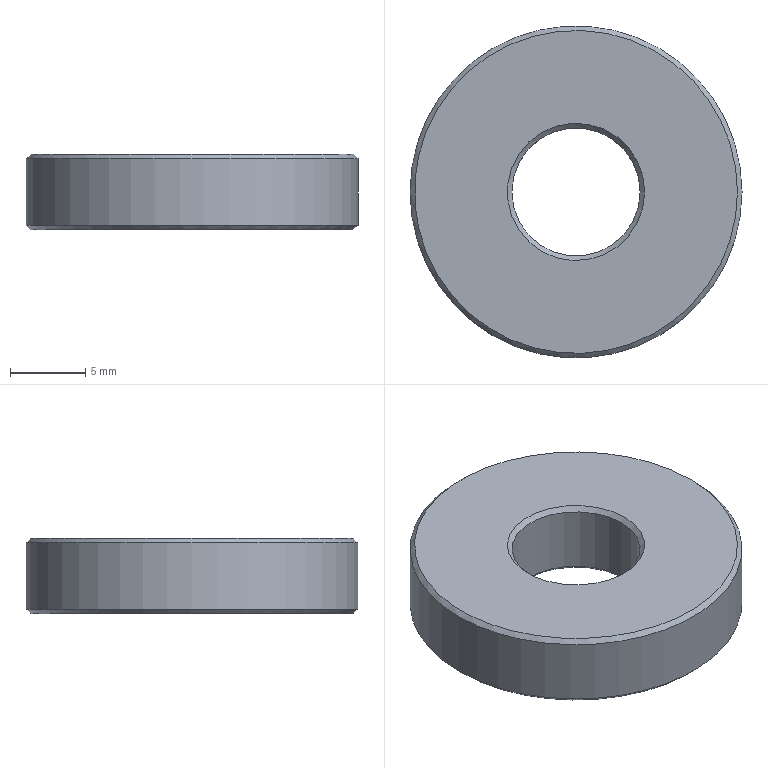Part | STEP file | 1 solid | 8 faces | box 22 x 22 x 5 mm | volume 1608 mm3 | cone 4 | plane 2 | cylinder 2 | commonest cylinder face diameters 8.5 x1 22 x1
STEP:
#1=CARTESIAN_POINT('',(0.,0.,0.));
#2=DIRECTION('',(0.,0.,1.));
#3=DIRECTION('',(1.,0.,0.));
#4=AXIS2_PLACEMENT_3D('',#1,#2,#3);
#5=CARTESIAN_POINT('',(1433.797,497.48,48.619));
#6=VERTEX_POINT('',#5);
#7=CARTESIAN_POINT('',(1429.247,497.48,48.619));
#8=DIRECTION('',(0.,0.,-1.));
#9=DIRECTION('',(1.,0.,0.));
#10=AXIS2_PLACEMENT_3D('',#7,#8,#9);
#11=CIRCLE('',#10,4.55);
#12=CARTESIAN_POINT('',(1429.247,497.48,48.619));
#13=DIRECTION('',(0.,0.,1.));
#14=DIRECTION('',(1.,0.,0.));
#15=AXIS2_PLACEMENT_3D('',#12,#13,#14);
#16=PLANE('',#15);
#17=CARTESIAN_POINT('',(4.55,0.));
#18=CARTESIAN_POINT('',(4.55,-7.881));
#19=CARTESIAN_POINT('',(-2.275,-3.94));
#20=CARTESIAN_POINT('',(-9.1,0.));
#21=CARTESIAN_POINT('',(-2.275,3.94));
#22=CARTESIAN_POINT('',(4.55,7.881));
#23=CARTESIAN_POINT('',(4.55,0.));
#24=(BOUNDED_CURVE()B_SPLINE_CURVE(2,(#17,#18,#19,#20,#21,#22,#23),.UNSPECIFIED.,.T.,.F.)B_SPLINE_CURVE_WITH_KNOTS((1,2,2,2,2,1),(-2.094,0.,2.094,4.189,6.283,8.378),.UNSPECIFIED.)CURVE()GEOMETRIC_REPRESENTATION_ITEM()RATIONAL_B_SPLINE_CURVE((1.,0.5,1.,0.5,1.,0.5,1.))REPRESENTATION_ITEM(''));
#25=(GEOMETRIC_REPRESENTATION_CONTEXT(2)PARAMETRIC_REPRESENTATION_CONTEXT()REPRESENTATION_CONTEXT('',''));
#26=DEFINITIONAL_REPRESENTATION('',(#24),#25);
#27=PCURVE('',#16,#26);
#28=CARTESIAN_POINT('',(1429.247,497.48,48.619));
#29=DIRECTION('',(0.,0.,1.));
#30=DIRECTION('',(1.,0.,0.));
#31=AXIS2_PLACEMENT_3D('',#28,#29,#30);
#32=CONICAL_SURFACE('',#31,4.55,0.7854);
#33=CARTESIAN_POINT('',(6.283,0.));
#34=DIRECTION('',(-1.,0.));
#35=VECTOR('',#34,1.);
#36=LINE('',#33,#35);
#37=(GEOMETRIC_REPRESENTATION_CONTEXT(2)PARAMETRIC_REPRESENTATION_CONTEXT()REPRESENTATION_CONTEXT('',''));
#38=DEFINITIONAL_REPRESENTATION('',(#36),#37);
#39=PCURVE('',#32,#38);
#40=SURFACE_CURVE('',#11,(#27,#39),.PCURVE_S1.);
#41=EDGE_CURVE('',#6,#6,#40,.T.);
#42=ORIENTED_EDGE('',*,*,#41,.T.);
#43=EDGE_LOOP('',(#42));
#44=FACE_BOUND('',#43,.T.);
#45=CARTESIAN_POINT('',(1439.947,497.48,48.619));
#46=VERTEX_POINT('',#45);
#47=CARTESIAN_POINT('',(1429.247,497.48,48.619));
#48=DIRECTION('',(0.,0.,1.));
#49=DIRECTION('',(1.,0.,0.));
#50=AXIS2_PLACEMENT_3D('',#47,#48,#49);
#51=CIRCLE('',#50,10.7);
#52=CARTESIAN_POINT('',(0.,0.));
#53=DIRECTION('',(1.,0.));
#54=AXIS2_PLACEMENT_2D('',#52,#53);
#55=CIRCLE('',#54,10.7);
#56=(GEOMETRIC_REPRESENTATION_CONTEXT(2)PARAMETRIC_REPRESENTATION_CONTEXT()REPRESENTATION_CONTEXT('',''));
#57=DEFINITIONAL_REPRESENTATION('',(#55),#56);
#58=PCURVE('',#16,#57);
#59=CARTESIAN_POINT('',(1429.247,497.48,48.619));
#60=DIRECTION('',(0.,0.,-1.));
#61=DIRECTION('',(-1.,0.,0.));
#62=AXIS2_PLACEMENT_3D('',#59,#60,#61);
#63=CONICAL_SURFACE('',#62,10.7,0.7854);
#64=CARTESIAN_POINT('',(9.425,0.));
#65=DIRECTION('',(-1.,0.));
#66=VECTOR('',#65,1.);
#67=LINE('',#64,#66);
#68=(GEOMETRIC_REPRESENTATION_CONTEXT(2)PARAMETRIC_REPRESENTATION_CONTEXT()REPRESENTATION_CONTEXT('',''));
#69=DEFINITIONAL_REPRESENTATION('',(#67),#68);
#70=PCURVE('',#63,#69);
#71=SURFACE_CURVE('',#51,(#58,#70),.PCURVE_S1.);
#72=EDGE_CURVE('',#46,#46,#71,.T.);
#73=ORIENTED_EDGE('',*,*,#72,.T.);
#74=EDGE_LOOP('',(#73));
#75=FACE_BOUND('',#74,.T.);
#76=ADVANCED_FACE('',(#44,#75),#16,.T.);
#77=CARTESIAN_POINT('',(1424.697,497.48,43.619));
#78=VERTEX_POINT('',#77);
#79=CARTESIAN_POINT('',(1429.247,497.48,43.619));
#80=DIRECTION('',(0.,0.,1.));
#81=DIRECTION('',(-1.,0.,0.));
#82=AXIS2_PLACEMENT_3D('',#79,#80,#81);
#83=CIRCLE('',#82,4.55);
#84=CARTESIAN_POINT('',(1429.247,497.48,43.619));
#85=DIRECTION('',(0.,0.,-1.));
#86=DIRECTION('',(-1.,0.,0.));
#87=AXIS2_PLACEMENT_3D('',#84,#85,#86);
#88=PLANE('',#87);
#89=CARTESIAN_POINT('',(4.55,0.));
#90=CARTESIAN_POINT('',(4.55,-7.881));
#91=CARTESIAN_POINT('',(-2.275,-3.94));
#92=CARTESIAN_POINT('',(-9.1,0.));
#93=CARTESIAN_POINT('',(-2.275,3.94));
#94=CARTESIAN_POINT('',(4.55,7.881));
#95=CARTESIAN_POINT('',(4.55,0.));
#96=(BOUNDED_CURVE()B_SPLINE_CURVE(2,(#89,#90,#91,#92,#93,#94,#95),.UNSPECIFIED.,.T.,.F.)B_SPLINE_CURVE_WITH_KNOTS((1,2,2,2,2,1),(-2.094,0.,2.094,4.189,6.283,8.378),.UNSPECIFIED.)CURVE()GEOMETRIC_REPRESENTATION_ITEM()RATIONAL_B_SPLINE_CURVE((1.,0.5,1.,0.5,1.,0.5,1.))REPRESENTATION_ITEM(''));
#97=(GEOMETRIC_REPRESENTATION_CONTEXT(2)PARAMETRIC_REPRESENTATION_CONTEXT()REPRESENTATION_CONTEXT('',''));
#98=DEFINITIONAL_REPRESENTATION('',(#96),#97);
#99=PCURVE('',#88,#98);
#100=CARTESIAN_POINT('',(1429.247,497.48,43.919));
#101=DIRECTION('',(0.,0.,-1.));
#102=DIRECTION('',(-1.,0.,0.));
#103=AXIS2_PLACEMENT_3D('',#100,#101,#102);
#104=CONICAL_SURFACE('',#103,4.25,0.7854);
#105=CARTESIAN_POINT('',(6.283,0.3));
#106=DIRECTION('',(-1.,0.));
#107=VECTOR('',#106,1.);
#108=LINE('',#105,#107);
#109=(GEOMETRIC_REPRESENTATION_CONTEXT(2)PARAMETRIC_REPRESENTATION_CONTEXT()REPRESENTATION_CONTEXT('',''));
#110=DEFINITIONAL_REPRESENTATION('',(#108),#109);
#111=PCURVE('',#104,#110);
#112=SURFACE_CURVE('',#83,(#99,#111),.PCURVE_S1.);
#113=EDGE_CURVE('',#78,#78,#112,.T.);
#114=ORIENTED_EDGE('',*,*,#113,.T.);
#115=EDGE_LOOP('',(#114));
#116=FACE_BOUND('',#115,.T.);
#117=CARTESIAN_POINT('',(1418.547,497.48,43.619));
#118=VERTEX_POINT('',#117);
#119=CARTESIAN_POINT('',(1429.247,497.48,43.619));
#120=DIRECTION('',(0.,0.,-1.));
#121=DIRECTION('',(-1.,0.,0.));
#122=AXIS2_PLACEMENT_3D('',#119,#120,#121);
#123=CIRCLE('',#122,10.7);
#124=CARTESIAN_POINT('',(0.,0.));
#125=DIRECTION('',(1.,0.));
#126=AXIS2_PLACEMENT_2D('',#124,#125);
#127=CIRCLE('',#126,10.7);
#128=(GEOMETRIC_REPRESENTATION_CONTEXT(2)PARAMETRIC_REPRESENTATION_CONTEXT()REPRESENTATION_CONTEXT('',''));
#129=DEFINITIONAL_REPRESENTATION('',(#127),#128);
#130=PCURVE('',#88,#129);
#131=CARTESIAN_POINT('',(1429.247,497.48,43.619));
#132=DIRECTION('',(0.,0.,1.));
#133=DIRECTION('',(1.,0.,0.));
#134=AXIS2_PLACEMENT_3D('',#131,#132,#133);
#135=CONICAL_SURFACE('',#134,10.7,0.7854);
#136=CARTESIAN_POINT('',(9.425,0.));
#137=DIRECTION('',(-1.,0.));
#138=VECTOR('',#137,1.);
#139=LINE('',#136,#138);
#140=(GEOMETRIC_REPRESENTATION_CONTEXT(2)PARAMETRIC_REPRESENTATION_CONTEXT()REPRESENTATION_CONTEXT('',''));
#141=DEFINITIONAL_REPRESENTATION('',(#139),#140);
#142=PCURVE('',#135,#141);
#143=SURFACE_CURVE('',#123,(#130,#142),.PCURVE_S1.);
#144=EDGE_CURVE('',#118,#118,#143,.T.);
#145=ORIENTED_EDGE('',*,*,#144,.T.);
#146=EDGE_LOOP('',(#145));
#147=FACE_BOUND('',#146,.T.);
#148=ADVANCED_FACE('',(#116,#147),#88,.T.);
#149=CARTESIAN_POINT('',(1440.247,497.48,48.319));
#150=VERTEX_POINT('',#149);
#151=CARTESIAN_POINT('',(1418.247,497.48,48.319));
#152=VERTEX_POINT('',#151);
#153=CARTESIAN_POINT('',(1429.247,497.48,48.319));
#154=DIRECTION('',(0.,0.,-1.));
#155=DIRECTION('',(1.,0.,0.));
#156=AXIS2_PLACEMENT_3D('',#153,#154,#155);
#157=CIRCLE('',#156,11.);
#158=CARTESIAN_POINT('',(1429.247,497.48,43.619));
#159=DIRECTION('',(0.,0.,1.));
#160=DIRECTION('',(-1.,0.,0.));
#161=AXIS2_PLACEMENT_3D('',#158,#159,#160);
#162=CYLINDRICAL_SURFACE('',#161,11.);
#163=CARTESIAN_POINT('',(3.142,4.7));
#164=DIRECTION('',(-1.,0.));
#165=VECTOR('',#164,1.);
#166=LINE('',#163,#165);
#167=(GEOMETRIC_REPRESENTATION_CONTEXT(2)PARAMETRIC_REPRESENTATION_CONTEXT()REPRESENTATION_CONTEXT('',''));
#168=DEFINITIONAL_REPRESENTATION('',(#166),#167);
#169=PCURVE('',#162,#168);
#170=CARTESIAN_POINT('',(3.142,0.3));
#171=DIRECTION('',(1.,0.));
#172=VECTOR('',#171,1.);
#173=LINE('',#170,#172);
#174=(GEOMETRIC_REPRESENTATION_CONTEXT(2)PARAMETRIC_REPRESENTATION_CONTEXT()REPRESENTATION_CONTEXT('',''));
#175=DEFINITIONAL_REPRESENTATION('',(#173),#174);
#176=PCURVE('',#63,#175);
#177=SURFACE_CURVE('',#157,(#169,#176),.PCURVE_S1.);
#178=EDGE_CURVE('',#150,#152,#177,.T.);
#179=ORIENTED_EDGE('',*,*,#178,.T.);
#180=CARTESIAN_POINT('',(1418.247,497.48,43.919));
#181=VERTEX_POINT('',#180);
#182=CARTESIAN_POINT('',(1418.247,497.48,43.919));
#183=CARTESIAN_POINT('',(1418.247,497.48,48.319));
#184=B_SPLINE_CURVE_WITH_KNOTS('',1,(#182,#183),.UNSPECIFIED.,.F.,.F.,(2,2),(0.3,4.7),.PIECEWISE_BEZIER_KNOTS.);
#185=CARTESIAN_POINT('',(0.,0.));
#186=DIRECTION('',(0.,1.));
#187=VECTOR('',#186,1.);
#188=LINE('',#185,#187);
#189=(GEOMETRIC_REPRESENTATION_CONTEXT(2)PARAMETRIC_REPRESENTATION_CONTEXT()REPRESENTATION_CONTEXT('',''));
#190=DEFINITIONAL_REPRESENTATION('',(#188),#189);
#191=PCURVE('',#162,#190);
#192=CARTESIAN_POINT('',(6.283,0.));
#193=DIRECTION('',(0.,1.));
#194=VECTOR('',#193,1.);
#195=LINE('',#192,#194);
#196=(GEOMETRIC_REPRESENTATION_CONTEXT(2)PARAMETRIC_REPRESENTATION_CONTEXT()REPRESENTATION_CONTEXT('',''));
#197=DEFINITIONAL_REPRESENTATION('',(#195),#196);
#198=PCURVE('',#162,#197);
#199=SEAM_CURVE('',#184,(#191,#198),.PCURVE_S1.);
#200=EDGE_CURVE('',#181,#152,#199,.T.);
#201=ORIENTED_EDGE('',*,*,#200,.F.);
#202=CARTESIAN_POINT('',(1429.247,497.48,43.919));
#203=DIRECTION('',(0.,0.,1.));
#204=DIRECTION('',(-1.,0.,0.));
#205=AXIS2_PLACEMENT_3D('',#202,#203,#204);
#206=CIRCLE('',#205,11.);
#207=CARTESIAN_POINT('',(0.,0.3));
#208=DIRECTION('',(1.,0.));
#209=VECTOR('',#208,1.);
#210=LINE('',#207,#209);
#211=(GEOMETRIC_REPRESENTATION_CONTEXT(2)PARAMETRIC_REPRESENTATION_CONTEXT()REPRESENTATION_CONTEXT('',''));
#212=DEFINITIONAL_REPRESENTATION('',(#210),#211);
#213=PCURVE('',#162,#212);
#214=CARTESIAN_POINT('',(3.142,0.3));
#215=DIRECTION('',(1.,0.));
#216=VECTOR('',#215,1.);
#217=LINE('',#214,#216);
#218=(GEOMETRIC_REPRESENTATION_CONTEXT(2)PARAMETRIC_REPRESENTATION_CONTEXT()REPRESENTATION_CONTEXT('',''));
#219=DEFINITIONAL_REPRESENTATION('',(#217),#218);
#220=PCURVE('',#135,#219);
#221=SURFACE_CURVE('',#206,(#213,#220),.PCURVE_S1.);
#222=EDGE_CURVE('',#181,#181,#221,.T.);
#223=ORIENTED_EDGE('',*,*,#222,.T.);
#224=ORIENTED_EDGE('',*,*,#200,.T.);
#225=CARTESIAN_POINT('',(1429.247,497.48,48.319));
#226=DIRECTION('',(0.,0.,-1.));
#227=DIRECTION('',(1.,0.,0.));
#228=AXIS2_PLACEMENT_3D('',#225,#226,#227);
#229=CIRCLE('',#228,11.);
#230=CARTESIAN_POINT('',(9.425,4.7));
#231=DIRECTION('',(-1.,0.));
#232=VECTOR('',#231,1.);
#233=LINE('',#230,#232);
#234=(GEOMETRIC_REPRESENTATION_CONTEXT(2)PARAMETRIC_REPRESENTATION_CONTEXT()REPRESENTATION_CONTEXT('',''));
#235=DEFINITIONAL_REPRESENTATION('',(#233),#234);
#236=PCURVE('',#162,#235);
#237=CARTESIAN_POINT('',(3.142,0.3));
#238=DIRECTION('',(1.,0.));
#239=VECTOR('',#238,1.);
#240=LINE('',#237,#239);
#241=(GEOMETRIC_REPRESENTATION_CONTEXT(2)PARAMETRIC_REPRESENTATION_CONTEXT()REPRESENTATION_CONTEXT('',''));
#242=DEFINITIONAL_REPRESENTATION('',(#240),#241);
#243=PCURVE('',#63,#242);
#244=SURFACE_CURVE('',#229,(#236,#243),.PCURVE_S1.);
#245=EDGE_CURVE('',#152,#150,#244,.T.);
#246=ORIENTED_EDGE('',*,*,#245,.T.);
#247=EDGE_LOOP('',(#179,#201,#223,#224,#246));
#248=FACE_BOUND('',#247,.T.);
#249=ADVANCED_FACE('',(#248),#162,.T.);
#250=CARTESIAN_POINT('',(1424.997,497.48,43.919));
#251=VERTEX_POINT('',#250);
#252=CARTESIAN_POINT('',(1429.247,497.48,43.919));
#253=DIRECTION('',(0.,0.,-1.));
#254=DIRECTION('',(-1.,0.,0.));
#255=AXIS2_PLACEMENT_3D('',#252,#253,#254);
#256=CIRCLE('',#255,4.25);
#257=CARTESIAN_POINT('',(1429.247,497.48,48.619));
#258=DIRECTION('',(0.,0.,-1.));
#259=DIRECTION('',(-1.,0.,0.));
#260=AXIS2_PLACEMENT_3D('',#257,#258,#259);
#261=CYLINDRICAL_SURFACE('',#260,4.25);
#262=CARTESIAN_POINT('',(0.,4.7));
#263=DIRECTION('',(1.,0.));
#264=VECTOR('',#263,1.);
#265=LINE('',#262,#264);
#266=(GEOMETRIC_REPRESENTATION_CONTEXT(2)PARAMETRIC_REPRESENTATION_CONTEXT()REPRESENTATION_CONTEXT('',''));
#267=DEFINITIONAL_REPRESENTATION('',(#265),#266);
#268=PCURVE('',#261,#267);
#269=CARTESIAN_POINT('',(0.,0.));
#270=DIRECTION('',(1.,0.));
#271=VECTOR('',#270,1.);
#272=LINE('',#269,#271);
#273=(GEOMETRIC_REPRESENTATION_CONTEXT(2)PARAMETRIC_REPRESENTATION_CONTEXT()REPRESENTATION_CONTEXT('',''));
#274=DEFINITIONAL_REPRESENTATION('',(#272),#273);
#275=PCURVE('',#104,#274);
#276=SURFACE_CURVE('',#256,(#268,#275),.PCURVE_S1.);
#277=EDGE_CURVE('',#251,#251,#276,.T.);
#278=ORIENTED_EDGE('',*,*,#277,.F.);
#279=CARTESIAN_POINT('',(1424.997,497.48,48.319));
#280=VERTEX_POINT('',#279);
#281=CARTESIAN_POINT('',(1424.997,497.48,48.319));
#282=CARTESIAN_POINT('',(1424.997,497.48,43.919));
#283=B_SPLINE_CURVE_WITH_KNOTS('',1,(#281,#282),.UNSPECIFIED.,.F.,.F.,(2,2),(0.3,4.7),.PIECEWISE_BEZIER_KNOTS.);
#284=CARTESIAN_POINT('',(0.,0.));
#285=DIRECTION('',(0.,1.));
#286=VECTOR('',#285,1.);
#287=LINE('',#284,#286);
#288=(GEOMETRIC_REPRESENTATION_CONTEXT(2)PARAMETRIC_REPRESENTATION_CONTEXT()REPRESENTATION_CONTEXT('',''));
#289=DEFINITIONAL_REPRESENTATION('',(#287),#288);
#290=PCURVE('',#261,#289);
#291=CARTESIAN_POINT('',(6.283,0.));
#292=DIRECTION('',(0.,1.));
#293=VECTOR('',#292,1.);
#294=LINE('',#291,#293);
#295=(GEOMETRIC_REPRESENTATION_CONTEXT(2)PARAMETRIC_REPRESENTATION_CONTEXT()REPRESENTATION_CONTEXT('',''));
#296=DEFINITIONAL_REPRESENTATION('',(#294),#295);
#297=PCURVE('',#261,#296);
#298=SEAM_CURVE('',#283,(#290,#297),.PCURVE_S1.);
#299=EDGE_CURVE('',#280,#251,#298,.T.);
#300=ORIENTED_EDGE('',*,*,#299,.F.);
#301=CARTESIAN_POINT('',(1433.497,497.48,48.319));
#302=VERTEX_POINT('',#301);
#303=CARTESIAN_POINT('',(1429.247,497.48,48.319));
#304=DIRECTION('',(0.,0.,1.));
#305=DIRECTION('',(1.,0.,0.));
#306=AXIS2_PLACEMENT_3D('',#303,#304,#305);
#307=CIRCLE('',#306,4.25);
#308=CARTESIAN_POINT('',(3.142,0.3));
#309=DIRECTION('',(-1.,0.));
#310=VECTOR('',#309,1.);
#311=LINE('',#308,#310);
#312=(GEOMETRIC_REPRESENTATION_CONTEXT(2)PARAMETRIC_REPRESENTATION_CONTEXT()REPRESENTATION_CONTEXT('',''));
#313=DEFINITIONAL_REPRESENTATION('',(#311),#312);
#314=PCURVE('',#261,#313);
#315=CARTESIAN_POINT('',(0.,-0.3));
#316=DIRECTION('',(1.,0.));
#317=VECTOR('',#316,1.);
#318=LINE('',#315,#317);
#319=(GEOMETRIC_REPRESENTATION_CONTEXT(2)PARAMETRIC_REPRESENTATION_CONTEXT()REPRESENTATION_CONTEXT('',''));
#320=DEFINITIONAL_REPRESENTATION('',(#318),#319);
#321=PCURVE('',#32,#320);
#322=SURFACE_CURVE('',#307,(#314,#321),.PCURVE_S1.);
#323=EDGE_CURVE('',#302,#280,#322,.T.);
#324=ORIENTED_EDGE('',*,*,#323,.F.);
#325=CARTESIAN_POINT('',(1429.247,497.48,48.319));
#326=DIRECTION('',(0.,0.,1.));
#327=DIRECTION('',(1.,0.,0.));
#328=AXIS2_PLACEMENT_3D('',#325,#326,#327);
#329=CIRCLE('',#328,4.25);
#330=CARTESIAN_POINT('',(9.425,0.3));
#331=DIRECTION('',(-1.,0.));
#332=VECTOR('',#331,1.);
#333=LINE('',#330,#332);
#334=(GEOMETRIC_REPRESENTATION_CONTEXT(2)PARAMETRIC_REPRESENTATION_CONTEXT()REPRESENTATION_CONTEXT('',''));
#335=DEFINITIONAL_REPRESENTATION('',(#333),#334);
#336=PCURVE('',#261,#335);
#337=CARTESIAN_POINT('',(0.,-0.3));
#338=DIRECTION('',(1.,0.));
#339=VECTOR('',#338,1.);
#340=LINE('',#337,#339);
#341=(GEOMETRIC_REPRESENTATION_CONTEXT(2)PARAMETRIC_REPRESENTATION_CONTEXT()REPRESENTATION_CONTEXT('',''));
#342=DEFINITIONAL_REPRESENTATION('',(#340),#341);
#343=PCURVE('',#32,#342);
#344=SURFACE_CURVE('',#329,(#336,#343),.PCURVE_S1.);
#345=EDGE_CURVE('',#280,#302,#344,.T.);
#346=ORIENTED_EDGE('',*,*,#345,.F.);
#347=ORIENTED_EDGE('',*,*,#299,.T.);
#348=EDGE_LOOP('',(#278,#300,#324,#346,#347));
#349=FACE_BOUND('',#348,.F.);
#350=ADVANCED_FACE('',(#349),#261,.F.);
#351=ORIENTED_EDGE('',*,*,#178,.F.);
#352=CARTESIAN_POINT('',(1439.947,497.48,48.619));
#353=CARTESIAN_POINT('',(1440.247,497.48,48.319));
#354=B_SPLINE_CURVE_WITH_KNOTS('',1,(#352,#353),.UNSPECIFIED.,.F.,.F.,(2,2),(0.,0.4243),.PIECEWISE_BEZIER_KNOTS.);
#355=CARTESIAN_POINT('',(3.142,0.));
#356=DIRECTION('',(0.,1.));
#357=VECTOR('',#356,1.);
#358=LINE('',#355,#357);
#359=(GEOMETRIC_REPRESENTATION_CONTEXT(2)PARAMETRIC_REPRESENTATION_CONTEXT()REPRESENTATION_CONTEXT('',''));
#360=DEFINITIONAL_REPRESENTATION('',(#358),#359);
#361=PCURVE('',#63,#360);
#362=CARTESIAN_POINT('',(9.425,0.));
#363=DIRECTION('',(0.,1.));
#364=VECTOR('',#363,1.);
#365=LINE('',#362,#364);
#366=(GEOMETRIC_REPRESENTATION_CONTEXT(2)PARAMETRIC_REPRESENTATION_CONTEXT()REPRESENTATION_CONTEXT('',''));
#367=DEFINITIONAL_REPRESENTATION('',(#365),#366);
#368=PCURVE('',#63,#367);
#369=SEAM_CURVE('',#354,(#361,#368),.PCURVE_S1.);
#370=EDGE_CURVE('',#46,#150,#369,.T.);
#371=ORIENTED_EDGE('',*,*,#370,.F.);
#372=ORIENTED_EDGE('',*,*,#72,.F.);
#373=ORIENTED_EDGE('',*,*,#370,.T.);
#374=ORIENTED_EDGE('',*,*,#245,.F.);
#375=EDGE_LOOP('',(#351,#371,#372,#373,#374));
#376=FACE_BOUND('',#375,.T.);
#377=ADVANCED_FACE('',(#376),#63,.T.);
#378=ORIENTED_EDGE('',*,*,#222,.F.);
#379=CARTESIAN_POINT('',(1418.547,497.48,43.619));
#380=CARTESIAN_POINT('',(1418.247,497.48,43.919));
#381=B_SPLINE_CURVE_WITH_KNOTS('',1,(#379,#380),.UNSPECIFIED.,.F.,.F.,(2,2),(0.,0.4243),.PIECEWISE_BEZIER_KNOTS.);
#382=CARTESIAN_POINT('',(3.142,0.));
#383=DIRECTION('',(0.,1.));
#384=VECTOR('',#383,1.);
#385=LINE('',#382,#384);
#386=(GEOMETRIC_REPRESENTATION_CONTEXT(2)PARAMETRIC_REPRESENTATION_CONTEXT()REPRESENTATION_CONTEXT('',''));
#387=DEFINITIONAL_REPRESENTATION('',(#385),#386);
#388=PCURVE('',#135,#387);
#389=CARTESIAN_POINT('',(9.425,0.));
#390=DIRECTION('',(0.,1.));
#391=VECTOR('',#390,1.);
#392=LINE('',#389,#391);
#393=(GEOMETRIC_REPRESENTATION_CONTEXT(2)PARAMETRIC_REPRESENTATION_CONTEXT()REPRESENTATION_CONTEXT('',''));
#394=DEFINITIONAL_REPRESENTATION('',(#392),#393);
#395=PCURVE('',#135,#394);
#396=SEAM_CURVE('',#381,(#388,#395),.PCURVE_S1.);
#397=EDGE_CURVE('',#118,#181,#396,.T.);
#398=ORIENTED_EDGE('',*,*,#397,.F.);
#399=ORIENTED_EDGE('',*,*,#144,.F.);
#400=ORIENTED_EDGE('',*,*,#397,.T.);
#401=EDGE_LOOP('',(#378,#398,#399,#400));
#402=FACE_BOUND('',#401,.T.);
#403=ADVANCED_FACE('',(#402),#135,.T.);
#404=ORIENTED_EDGE('',*,*,#113,.T.);
#405=CARTESIAN_POINT('',(1424.997,497.48,43.919));
#406=CARTESIAN_POINT('',(1424.697,497.48,43.619));
#407=B_SPLINE_CURVE_WITH_KNOTS('',1,(#405,#406),.UNSPECIFIED.,.F.,.F.,(2,2),(0.,0.4243),.PIECEWISE_BEZIER_KNOTS.);
#408=CARTESIAN_POINT('',(0.,0.));
#409=DIRECTION('',(0.,1.));
#410=VECTOR('',#409,1.);
#411=LINE('',#408,#410);
#412=(GEOMETRIC_REPRESENTATION_CONTEXT(2)PARAMETRIC_REPRESENTATION_CONTEXT()REPRESENTATION_CONTEXT('',''));
#413=DEFINITIONAL_REPRESENTATION('',(#411),#412);
#414=PCURVE('',#104,#413);
#415=CARTESIAN_POINT('',(6.283,0.));
#416=DIRECTION('',(0.,1.));
#417=VECTOR('',#416,1.);
#418=LINE('',#415,#417);
#419=(GEOMETRIC_REPRESENTATION_CONTEXT(2)PARAMETRIC_REPRESENTATION_CONTEXT()REPRESENTATION_CONTEXT('',''));
#420=DEFINITIONAL_REPRESENTATION('',(#418),#419);
#421=PCURVE('',#104,#420);
#422=SEAM_CURVE('',#407,(#414,#421),.PCURVE_S1.);
#423=EDGE_CURVE('',#251,#78,#422,.T.);
#424=ORIENTED_EDGE('',*,*,#423,.F.);
#425=ORIENTED_EDGE('',*,*,#277,.T.);
#426=ORIENTED_EDGE('',*,*,#423,.T.);
#427=EDGE_LOOP('',(#404,#424,#425,#426));
#428=FACE_BOUND('',#427,.F.);
#429=ADVANCED_FACE('',(#428),#104,.F.);
#430=ORIENTED_EDGE('',*,*,#345,.T.);
#431=CARTESIAN_POINT('',(1433.497,497.48,48.319));
#432=CARTESIAN_POINT('',(1433.797,497.48,48.619));
#433=B_SPLINE_CURVE_WITH_KNOTS('',1,(#431,#432),.UNSPECIFIED.,.F.,.F.,(2,2),(-0.4243,0.),.PIECEWISE_BEZIER_KNOTS.);
#434=CARTESIAN_POINT('',(6.283,0.));
#435=DIRECTION('',(0.,1.));
#436=VECTOR('',#435,1.);
#437=LINE('',#434,#436);
#438=(GEOMETRIC_REPRESENTATION_CONTEXT(2)PARAMETRIC_REPRESENTATION_CONTEXT()REPRESENTATION_CONTEXT('',''));
#439=DEFINITIONAL_REPRESENTATION('',(#437),#438);
#440=PCURVE('',#32,#439);
#441=CARTESIAN_POINT('',(0.,0.));
#442=DIRECTION('',(0.,1.));
#443=VECTOR('',#442,1.);
#444=LINE('',#441,#443);
#445=(GEOMETRIC_REPRESENTATION_CONTEXT(2)PARAMETRIC_REPRESENTATION_CONTEXT()REPRESENTATION_CONTEXT('',''));
#446=DEFINITIONAL_REPRESENTATION('',(#444),#445);
#447=PCURVE('',#32,#446);
#448=SEAM_CURVE('',#433,(#440,#447),.PCURVE_S1.);
#449=EDGE_CURVE('',#302,#6,#448,.T.);
#450=ORIENTED_EDGE('',*,*,#449,.T.);
#451=ORIENTED_EDGE('',*,*,#41,.T.);
#452=ORIENTED_EDGE('',*,*,#449,.F.);
#453=ORIENTED_EDGE('',*,*,#323,.T.);
#454=EDGE_LOOP('',(#430,#450,#451,#452,#453));
#455=FACE_BOUND('',#454,.F.);
#456=ADVANCED_FACE('',(#455),#32,.F.);
#457=CLOSED_SHELL('',(#76,#148,#249,#350,#377,#403,#429,#456));
#458=MANIFOLD_SOLID_BREP('',#457);
#459=(LENGTH_UNIT()NAMED_UNIT(*)SI_UNIT(.MILLI.,.METRE.));
#460=UNCERTAINTY_MEASURE_WITH_UNIT(LENGTH_MEASURE(0.00001),#459,'','');
#461=(NAMED_UNIT(*)PLANE_ANGLE_UNIT()SI_UNIT($,.RADIAN.));
#462=(NAMED_UNIT(*)SI_UNIT($,.STERADIAN.)SOLID_ANGLE_UNIT());
#463=(GEOMETRIC_REPRESENTATION_CONTEXT(3)GLOBAL_UNCERTAINTY_ASSIGNED_CONTEXT((#460))GLOBAL_UNIT_ASSIGNED_CONTEXT((#459,#461,#462))REPRESENTATION_CONTEXT('',''));
#464=ADVANCED_BREP_SHAPE_REPRESENTATION('',(#4,#458),#463);